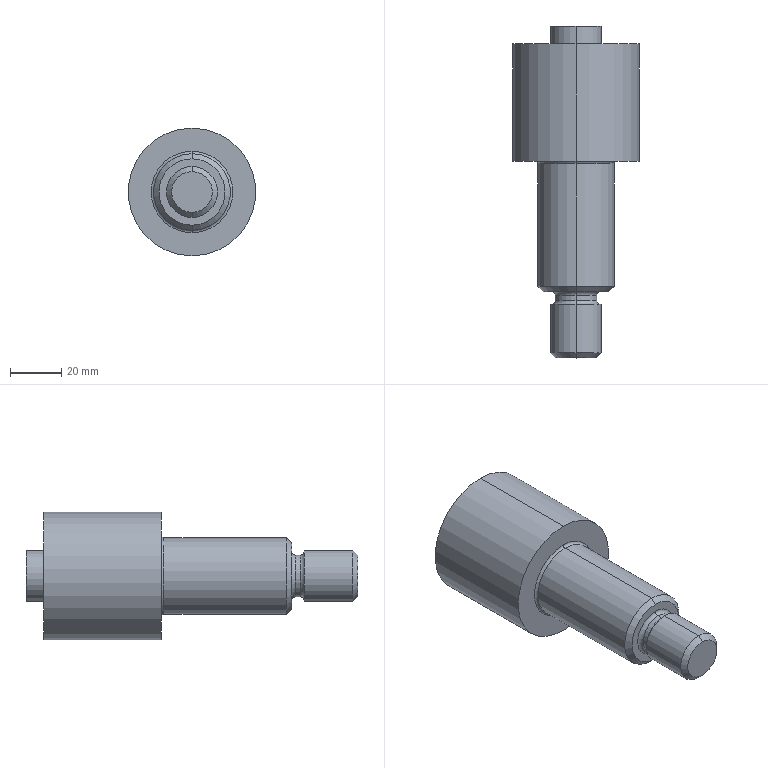Part | SolidWorks | features MirrorStock 1 | 1 solid | 26 faces | box 50 x 130 x 50 mm | volume 135954 mm3 | cylinder 10 | torus 6 | plane 6 | cone 4 | commonest cylinder face diameters 16.4 x2 19.8 x2 20 x2 30 x2 50 x2
STEP:
#1=CARTESIAN_POINT('',(0.,-107.5,-8.2));
#2=VERTEX_POINT('',#1);
#3=CARTESIAN_POINT('',(0.,-107.5,8.2));
#4=VERTEX_POINT('',#3);
#5=CARTESIAN_POINT('',(0.,-107.5,0.));
#6=DIRECTION('',(0.,-1.,0.));
#7=DIRECTION('',(0.,0.,-1.));
#8=AXIS2_PLACEMENT_3D('',#5,#6,#7);
#9=CIRCLE('',#8,8.2);
#10=EDGE_CURVE('',#2,#4,#9,.T.);
#11=ORIENTED_EDGE('',*,*,#10,.T.);
#12=CARTESIAN_POINT('',(0.,-109.,9.7));
#13=VERTEX_POINT('',#12);
#14=CARTESIAN_POINT('',(0.,-107.5,9.7));
#15=DIRECTION('',(-1.,0.,0.));
#16=DIRECTION('',(0.,0.,1.));
#17=AXIS2_PLACEMENT_3D('',#14,#15,#16);
#18=CIRCLE('',#17,1.5);
#19=EDGE_CURVE('',#4,#13,#18,.T.);
#20=ORIENTED_EDGE('',*,*,#19,.T.);
#21=CARTESIAN_POINT('',(0.,-109.,-9.7));
#22=VERTEX_POINT('',#21);
#23=CARTESIAN_POINT('',(0.,-109.,0.));
#24=DIRECTION('',(0.,1.,0.));
#25=DIRECTION('',(0.,0.,-1.));
#26=AXIS2_PLACEMENT_3D('',#23,#24,#25);
#27=CIRCLE('',#26,9.7);
#28=EDGE_CURVE('',#13,#22,#27,.T.);
#29=ORIENTED_EDGE('',*,*,#28,.T.);
#30=CARTESIAN_POINT('',(0.,-107.5,-9.7));
#31=DIRECTION('',(1.,0.,0.));
#32=DIRECTION('',(0.,0.,-1.));
#33=AXIS2_PLACEMENT_3D('',#30,#31,#32);
#34=CIRCLE('',#33,1.5);
#35=EDGE_CURVE('',#2,#22,#34,.T.);
#36=ORIENTED_EDGE('',*,*,#35,.F.);
#37=EDGE_LOOP('',(#11,#20,#29,#36));
#38=FACE_OUTER_BOUND('',#37,.T.);
#39=CARTESIAN_POINT('',(0.,-107.5,0.));
#40=DIRECTION('',(0.,1.,0.));
#41=DIRECTION('',(0.,0.,-1.));
#42=AXIS2_PLACEMENT_3D('',#39,#40,#41);
#43=TOROIDAL_SURFACE('',#42,9.7,1.5);
#44=ADVANCED_FACE('',(#38),#43,.F.);
#45=CARTESIAN_POINT('',(0.,-105.5,8.2));
#46=VERTEX_POINT('',#45);
#47=CARTESIAN_POINT('',(0.,-105.5,-8.2));
#48=VERTEX_POINT('',#47);
#49=CARTESIAN_POINT('',(0.,-105.5,0.));
#50=DIRECTION('',(0.,1.,0.));
#51=DIRECTION('',(0.,0.,1.));
#52=AXIS2_PLACEMENT_3D('',#49,#50,#51);
#53=CIRCLE('',#52,8.2);
#54=EDGE_CURVE('',#46,#48,#53,.T.);
#55=ORIENTED_EDGE('',*,*,#54,.T.);
#56=CARTESIAN_POINT('',(0.,-104.,-9.7));
#57=VERTEX_POINT('',#56);
#58=CARTESIAN_POINT('',(0.,-105.5,-9.7));
#59=DIRECTION('',(-1.,0.,0.));
#60=DIRECTION('',(0.,0.,1.));
#61=AXIS2_PLACEMENT_3D('',#58,#59,#60);
#62=CIRCLE('',#61,1.5);
#63=EDGE_CURVE('',#48,#57,#62,.T.);
#64=ORIENTED_EDGE('',*,*,#63,.T.);
#65=CARTESIAN_POINT('',(0.,-104.,9.7));
#66=VERTEX_POINT('',#65);
#67=CARTESIAN_POINT('',(0.,-104.,0.));
#68=DIRECTION('',(0.,-1.,0.));
#69=DIRECTION('',(0.,0.,1.));
#70=AXIS2_PLACEMENT_3D('',#67,#68,#69);
#71=CIRCLE('',#70,9.7);
#72=EDGE_CURVE('',#57,#66,#71,.T.);
#73=ORIENTED_EDGE('',*,*,#72,.T.);
#74=CARTESIAN_POINT('',(0.,-105.5,9.7));
#75=DIRECTION('',(1.,0.,0.));
#76=DIRECTION('',(0.,0.,-1.));
#77=AXIS2_PLACEMENT_3D('',#74,#75,#76);
#78=CIRCLE('',#77,1.5);
#79=EDGE_CURVE('',#46,#66,#78,.T.);
#80=ORIENTED_EDGE('',*,*,#79,.F.);
#81=EDGE_LOOP('',(#55,#64,#73,#80));
#82=FACE_OUTER_BOUND('',#81,.T.);
#83=CARTESIAN_POINT('',(0.,-105.5,0.));
#84=DIRECTION('',(0.,-1.,0.));
#85=DIRECTION('',(0.,0.,1.));
#86=AXIS2_PLACEMENT_3D('',#83,#84,#85);
#87=TOROIDAL_SURFACE('',#86,9.7,1.5);
#88=ADVANCED_FACE('',(#82),#87,.F.);
#89=CARTESIAN_POINT('',(0.,-54.,15.));
#90=VERTEX_POINT('',#89);
#91=CARTESIAN_POINT('',(0.,-54.,-15.));
#92=VERTEX_POINT('',#91);
#93=CARTESIAN_POINT('',(0.,-54.,0.));
#94=DIRECTION('',(0.,1.,0.));
#95=DIRECTION('',(0.,0.,1.));
#96=AXIS2_PLACEMENT_3D('',#93,#94,#95);
#97=CIRCLE('',#96,15.);
#98=EDGE_CURVE('',#90,#92,#97,.T.);
#99=ORIENTED_EDGE('',*,*,#98,.T.);
#100=CARTESIAN_POINT('',(0.,-53.,-16.));
#101=VERTEX_POINT('',#100);
#102=CARTESIAN_POINT('',(0.,-54.,-16.));
#103=DIRECTION('',(-1.,0.,0.));
#104=DIRECTION('',(0.,0.,1.));
#105=AXIS2_PLACEMENT_3D('',#102,#103,#104);
#106=CIRCLE('',#105,1.);
#107=EDGE_CURVE('',#92,#101,#106,.T.);
#108=ORIENTED_EDGE('',*,*,#107,.T.);
#109=CARTESIAN_POINT('',(0.,-53.,16.));
#110=VERTEX_POINT('',#109);
#111=CARTESIAN_POINT('',(0.,-53.,0.));
#112=DIRECTION('',(0.,-1.,0.));
#113=DIRECTION('',(0.,0.,1.));
#114=AXIS2_PLACEMENT_3D('',#111,#112,#113);
#115=CIRCLE('',#114,16.);
#116=EDGE_CURVE('',#101,#110,#115,.T.);
#117=ORIENTED_EDGE('',*,*,#116,.T.);
#118=CARTESIAN_POINT('',(0.,-54.,16.));
#119=DIRECTION('',(1.,0.,0.));
#120=DIRECTION('',(0.,0.,-1.));
#121=AXIS2_PLACEMENT_3D('',#118,#119,#120);
#122=CIRCLE('',#121,1.);
#123=EDGE_CURVE('',#90,#110,#122,.T.);
#124=ORIENTED_EDGE('',*,*,#123,.F.);
#125=EDGE_LOOP('',(#99,#108,#117,#124));
#126=FACE_OUTER_BOUND('',#125,.T.);
#127=CARTESIAN_POINT('',(0.,-54.,0.));
#128=DIRECTION('',(0.,-1.,0.));
#129=DIRECTION('',(0.,0.,1.));
#130=AXIS2_PLACEMENT_3D('',#127,#128,#129);
#131=TOROIDAL_SURFACE('',#130,16.,1.);
#132=ADVANCED_FACE('',(#126),#131,.F.);
#133=CARTESIAN_POINT('',(0.,-130.,-8.));
#134=VERTEX_POINT('',#133);
#135=CARTESIAN_POINT('',(0.,-130.,8.));
#136=VERTEX_POINT('',#135);
#137=CARTESIAN_POINT('',(0.,-130.,0.));
#138=DIRECTION('',(0.,1.,0.));
#139=DIRECTION('',(0.,0.,1.));
#140=AXIS2_PLACEMENT_3D('',#137,#138,#139);
#141=CIRCLE('',#140,8.);
#142=EDGE_CURVE('',#134,#136,#141,.T.);
#143=ORIENTED_EDGE('',*,*,#142,.T.);
#144=CARTESIAN_POINT('',(0.,-128.,10.));
#145=VERTEX_POINT('',#144);
#146=CARTESIAN_POINT('',(0.,-130.,8.));
#147=DIRECTION('',(0.,0.7071,0.7071));
#148=VECTOR('',#147,1000.);
#149=LINE('',#146,#148);
#150=EDGE_CURVE('',#136,#145,#149,.T.);
#151=ORIENTED_EDGE('',*,*,#150,.T.);
#152=CARTESIAN_POINT('',(0.,-128.,-10.));
#153=VERTEX_POINT('',#152);
#154=CARTESIAN_POINT('',(0.,-128.,0.));
#155=DIRECTION('',(0.,-1.,0.));
#156=DIRECTION('',(0.,0.,1.));
#157=AXIS2_PLACEMENT_3D('',#154,#155,#156);
#158=CIRCLE('',#157,10.);
#159=EDGE_CURVE('',#145,#153,#158,.T.);
#160=ORIENTED_EDGE('',*,*,#159,.T.);
#161=CARTESIAN_POINT('',(0.,-130.,-8.));
#162=DIRECTION('',(0.,0.7071,-0.7071));
#163=VECTOR('',#162,1000.);
#164=LINE('',#161,#163);
#165=EDGE_CURVE('',#134,#153,#164,.T.);
#166=ORIENTED_EDGE('',*,*,#165,.F.);
#167=EDGE_LOOP('',(#143,#151,#160,#166));
#168=FACE_OUTER_BOUND('',#167,.T.);
#169=CARTESIAN_POINT('',(0.,-130.,0.));
#170=DIRECTION('',(0.,1.,0.));
#171=DIRECTION('',(0.,0.,-1.));
#172=AXIS2_PLACEMENT_3D('',#169,#170,#171);
#173=CONICAL_SURFACE('',#172,8.,0.7854);
#174=ADVANCED_FACE('',(#168),#173,.T.);
#175=CARTESIAN_POINT('',(0.,-104.,-13.));
#176=VERTEX_POINT('',#175);
#177=CARTESIAN_POINT('',(0.,-104.,13.));
#178=VERTEX_POINT('',#177);
#179=CARTESIAN_POINT('',(0.,-104.,0.));
#180=DIRECTION('',(0.,1.,0.));
#181=DIRECTION('',(0.,0.,1.));
#182=AXIS2_PLACEMENT_3D('',#179,#180,#181);
#183=CIRCLE('',#182,13.);
#184=EDGE_CURVE('',#176,#178,#183,.T.);
#185=ORIENTED_EDGE('',*,*,#184,.T.);
#186=CARTESIAN_POINT('',(0.,-102.,15.));
#187=VERTEX_POINT('',#186);
#188=CARTESIAN_POINT('',(0.,-104.,13.));
#189=DIRECTION('',(0.,0.7071,0.7071));
#190=VECTOR('',#189,1000.);
#191=LINE('',#188,#190);
#192=EDGE_CURVE('',#178,#187,#191,.T.);
#193=ORIENTED_EDGE('',*,*,#192,.T.);
#194=CARTESIAN_POINT('',(0.,-102.,-15.));
#195=VERTEX_POINT('',#194);
#196=CARTESIAN_POINT('',(0.,-102.,0.));
#197=DIRECTION('',(0.,-1.,0.));
#198=DIRECTION('',(0.,0.,1.));
#199=AXIS2_PLACEMENT_3D('',#196,#197,#198);
#200=CIRCLE('',#199,15.);
#201=EDGE_CURVE('',#187,#195,#200,.T.);
#202=ORIENTED_EDGE('',*,*,#201,.T.);
#203=CARTESIAN_POINT('',(0.,-104.,-13.));
#204=DIRECTION('',(0.,0.7071,-0.7071));
#205=VECTOR('',#204,1000.);
#206=LINE('',#203,#205);
#207=EDGE_CURVE('',#176,#195,#206,.T.);
#208=ORIENTED_EDGE('',*,*,#207,.F.);
#209=EDGE_LOOP('',(#185,#193,#202,#208));
#210=FACE_OUTER_BOUND('',#209,.T.);
#211=CARTESIAN_POINT('',(0.,-104.,0.));
#212=DIRECTION('',(0.,1.,0.));
#213=DIRECTION('',(0.,0.,-1.));
#214=AXIS2_PLACEMENT_3D('',#211,#212,#213);
#215=CONICAL_SURFACE('',#214,13.,0.7854);
#216=ADVANCED_FACE('',(#210),#215,.T.);
#217=CARTESIAN_POINT('',(0.,-109.,-10.));
#218=VERTEX_POINT('',#217);
#219=CARTESIAN_POINT('',(0.,-109.,10.));
#220=VERTEX_POINT('',#219);
#221=CARTESIAN_POINT('',(0.,-109.,0.));
#222=DIRECTION('',(0.,1.,0.));
#223=DIRECTION('',(0.,0.,1.));
#224=AXIS2_PLACEMENT_3D('',#221,#222,#223);
#225=CIRCLE('',#224,10.);
#226=EDGE_CURVE('',#218,#220,#225,.T.);
#227=ORIENTED_EDGE('',*,*,#226,.F.);
#228=CARTESIAN_POINT('',(0.,-130.,-10.));
#229=DIRECTION('',(0.,-1.,0.));
#230=VECTOR('',#229,1000.);
#231=LINE('',#228,#230);
#232=EDGE_CURVE('',#218,#153,#231,.T.);
#233=ORIENTED_EDGE('',*,*,#232,.T.);
#234=ORIENTED_EDGE('',*,*,#159,.F.);
#235=CARTESIAN_POINT('',(0.,-130.,10.));
#236=DIRECTION('',(0.,-1.,0.));
#237=VECTOR('',#236,1000.);
#238=LINE('',#235,#237);
#239=EDGE_CURVE('',#220,#145,#238,.T.);
#240=ORIENTED_EDGE('',*,*,#239,.F.);
#241=EDGE_LOOP('',(#227,#233,#234,#240));
#242=FACE_OUTER_BOUND('',#241,.T.);
#243=CARTESIAN_POINT('',(0.,-130.,0.));
#244=DIRECTION('',(0.,-1.,0.));
#245=DIRECTION('',(0.,0.,1.));
#246=AXIS2_PLACEMENT_3D('',#243,#244,#245);
#247=CYLINDRICAL_SURFACE('',#246,10.);
#248=ADVANCED_FACE('',(#242),#247,.T.);
#249=CARTESIAN_POINT('',(0.,-105.5,0.));
#250=DIRECTION('',(0.,1.,0.));
#251=DIRECTION('',(0.,0.,1.));
#252=AXIS2_PLACEMENT_3D('',#249,#250,#251);
#253=CIRCLE('',#252,8.2);
#254=EDGE_CURVE('',#48,#46,#253,.T.);
#255=ORIENTED_EDGE('',*,*,#254,.F.);
#256=CARTESIAN_POINT('',(0.,-130.,-8.2));
#257=DIRECTION('',(0.,-1.,0.));
#258=VECTOR('',#257,1000.);
#259=LINE('',#256,#258);
#260=EDGE_CURVE('',#48,#2,#259,.T.);
#261=ORIENTED_EDGE('',*,*,#260,.T.);
#262=CARTESIAN_POINT('',(0.,-107.5,0.));
#263=DIRECTION('',(0.,-1.,0.));
#264=DIRECTION('',(0.,0.,-1.));
#265=AXIS2_PLACEMENT_3D('',#262,#263,#264);
#266=CIRCLE('',#265,8.2);
#267=EDGE_CURVE('',#4,#2,#266,.T.);
#268=ORIENTED_EDGE('',*,*,#267,.F.);
#269=CARTESIAN_POINT('',(0.,-130.,8.2));
#270=DIRECTION('',(0.,-1.,0.));
#271=VECTOR('',#270,1000.);
#272=LINE('',#269,#271);
#273=EDGE_CURVE('',#46,#4,#272,.T.);
#274=ORIENTED_EDGE('',*,*,#273,.F.);
#275=EDGE_LOOP('',(#255,#261,#268,#274));
#276=FACE_OUTER_BOUND('',#275,.T.);
#277=CARTESIAN_POINT('',(0.,-130.,0.));
#278=DIRECTION('',(0.,-1.,0.));
#279=DIRECTION('',(0.,0.,1.));
#280=AXIS2_PLACEMENT_3D('',#277,#278,#279);
#281=CYLINDRICAL_SURFACE('',#280,8.2);
#282=ADVANCED_FACE('',(#276),#281,.T.);
#283=CARTESIAN_POINT('',(0.,-54.,0.));
#284=DIRECTION('',(0.,1.,0.));
#285=DIRECTION('',(0.,0.,1.));
#286=AXIS2_PLACEMENT_3D('',#283,#284,#285);
#287=CIRCLE('',#286,15.);
#288=EDGE_CURVE('',#92,#90,#287,.T.);
#289=ORIENTED_EDGE('',*,*,#288,.F.);
#290=CARTESIAN_POINT('',(0.,-130.,-15.));
#291=DIRECTION('',(0.,-1.,0.));
#292=VECTOR('',#291,1000.);
#293=LINE('',#290,#292);
#294=EDGE_CURVE('',#92,#195,#293,.T.);
#295=ORIENTED_EDGE('',*,*,#294,.T.);
#296=ORIENTED_EDGE('',*,*,#201,.F.);
#297=CARTESIAN_POINT('',(0.,-130.,15.));
#298=DIRECTION('',(0.,-1.,0.));
#299=VECTOR('',#298,1000.);
#300=LINE('',#297,#299);
#301=EDGE_CURVE('',#90,#187,#300,.T.);
#302=ORIENTED_EDGE('',*,*,#301,.F.);
#303=EDGE_LOOP('',(#289,#295,#296,#302));
#304=FACE_OUTER_BOUND('',#303,.T.);
#305=CARTESIAN_POINT('',(0.,-130.,0.));
#306=DIRECTION('',(0.,-1.,0.));
#307=DIRECTION('',(0.,0.,1.));
#308=AXIS2_PLACEMENT_3D('',#305,#306,#307);
#309=CYLINDRICAL_SURFACE('',#308,15.);
#310=ADVANCED_FACE('',(#304),#309,.T.);
#311=CARTESIAN_POINT('',(0.,-7.,-25.));
#312=VERTEX_POINT('',#311);
#313=CARTESIAN_POINT('',(0.,-7.,25.));
#314=VERTEX_POINT('',#313);
#315=CARTESIAN_POINT('',(0.,-7.,0.));
#316=DIRECTION('',(0.,1.,0.));
#317=DIRECTION('',(0.,0.,1.));
#318=AXIS2_PLACEMENT_3D('',#315,#316,#317);
#319=CIRCLE('',#318,25.);
#320=EDGE_CURVE('',#312,#314,#319,.T.);
#321=ORIENTED_EDGE('',*,*,#320,.F.);
#322=CARTESIAN_POINT('',(0.,-53.,-25.));
#323=VERTEX_POINT('',#322);
#324=CARTESIAN_POINT('',(0.,-130.,-25.));
#325=DIRECTION('',(0.,-1.,0.));
#326=VECTOR('',#325,1000.);
#327=LINE('',#324,#326);
#328=EDGE_CURVE('',#312,#323,#327,.T.);
#329=ORIENTED_EDGE('',*,*,#328,.T.);
#330=CARTESIAN_POINT('',(0.,-53.,25.));
#331=VERTEX_POINT('',#330);
#332=CARTESIAN_POINT('',(0.,-53.,0.));
#333=DIRECTION('',(0.,1.,0.));
#334=DIRECTION('',(0.,0.,1.));
#335=AXIS2_PLACEMENT_3D('',#332,#333,#334);
#336=CIRCLE('',#335,25.);
#337=EDGE_CURVE('',#323,#331,#336,.T.);
#338=ORIENTED_EDGE('',*,*,#337,.T.);
#339=CARTESIAN_POINT('',(0.,-130.,25.));
#340=DIRECTION('',(0.,-1.,0.));
#341=VECTOR('',#340,1000.);
#342=LINE('',#339,#341);
#343=EDGE_CURVE('',#314,#331,#342,.T.);
#344=ORIENTED_EDGE('',*,*,#343,.F.);
#345=EDGE_LOOP('',(#321,#329,#338,#344));
#346=FACE_OUTER_BOUND('',#345,.T.);
#347=CARTESIAN_POINT('',(0.,-130.,0.));
#348=DIRECTION('',(0.,-1.,0.));
#349=DIRECTION('',(0.,0.,1.));
#350=AXIS2_PLACEMENT_3D('',#347,#348,#349);
#351=CYLINDRICAL_SURFACE('',#350,25.);
#352=ADVANCED_FACE('',(#346),#351,.T.);
#353=CARTESIAN_POINT('',(0.,0.,-9.9));
#354=VERTEX_POINT('',#353);
#355=CARTESIAN_POINT('',(0.,0.,9.9));
#356=VERTEX_POINT('',#355);
#357=CARTESIAN_POINT('',(0.,0.,0.));
#358=DIRECTION('',(0.,1.,0.));
#359=DIRECTION('',(0.,0.,1.));
#360=AXIS2_PLACEMENT_3D('',#357,#358,#359);
#361=CIRCLE('',#360,9.9);
#362=EDGE_CURVE('',#354,#356,#361,.T.);
#363=ORIENTED_EDGE('',*,*,#362,.F.);
#364=CARTESIAN_POINT('',(0.,-7.,-9.9));
#365=VERTEX_POINT('',#364);
#366=CARTESIAN_POINT('',(0.,-130.,-9.9));
#367=DIRECTION('',(0.,-1.,0.));
#368=VECTOR('',#367,1000.);
#369=LINE('',#366,#368);
#370=EDGE_CURVE('',#354,#365,#369,.T.);
#371=ORIENTED_EDGE('',*,*,#370,.T.);
#372=CARTESIAN_POINT('',(0.,-7.,9.9));
#373=VERTEX_POINT('',#372);
#374=CARTESIAN_POINT('',(0.,-7.,0.));
#375=DIRECTION('',(0.,1.,0.));
#376=DIRECTION('',(0.,0.,1.));
#377=AXIS2_PLACEMENT_3D('',#374,#375,#376);
#378=CIRCLE('',#377,9.9);
#379=EDGE_CURVE('',#365,#373,#378,.T.);
#380=ORIENTED_EDGE('',*,*,#379,.T.);
#381=CARTESIAN_POINT('',(0.,-130.,9.9));
#382=DIRECTION('',(0.,-1.,0.));
#383=VECTOR('',#382,1000.);
#384=LINE('',#381,#383);
#385=EDGE_CURVE('',#356,#373,#384,.T.);
#386=ORIENTED_EDGE('',*,*,#385,.F.);
#387=EDGE_LOOP('',(#363,#371,#380,#386));
#388=FACE_OUTER_BOUND('',#387,.T.);
#389=CARTESIAN_POINT('',(0.,-130.,0.));
#390=DIRECTION('',(0.,-1.,0.));
#391=DIRECTION('',(0.,0.,1.));
#392=AXIS2_PLACEMENT_3D('',#389,#390,#391);
#393=CYLINDRICAL_SURFACE('',#392,9.9);
#394=ADVANCED_FACE('',(#388),#393,.T.);
#395=CARTESIAN_POINT('',(0.,0.,0.));
#396=DIRECTION('',(0.,1.,0.));
#397=DIRECTION('',(0.,0.,1.));
#398=AXIS2_PLACEMENT_3D('',#395,#396,#397);
#399=CIRCLE('',#398,9.9);
#400=EDGE_CURVE('',#356,#354,#399,.T.);
#401=ORIENTED_EDGE('',*,*,#400,.T.);
#402=ORIENTED_EDGE('',*,*,#362,.T.);
#403=EDGE_LOOP('',(#401,#402));
#404=FACE_OUTER_BOUND('',#403,.T.);
#405=CARTESIAN_POINT('',(0.,0.,0.));
#406=DIRECTION('',(0.,1.,0.));
#407=DIRECTION('',(0.,0.,-1.));
#408=AXIS2_PLACEMENT_3D('',#405,#406,#407);
#409=PLANE('',#408);
#410=ADVANCED_FACE('',(#404),#409,.T.);
#411=ORIENTED_EDGE('',*,*,#370,.F.);
#412=ORIENTED_EDGE('',*,*,#400,.F.);
#413=ORIENTED_EDGE('',*,*,#385,.T.);
#414=CARTESIAN_POINT('',(0.,-7.,0.));
#415=DIRECTION('',(0.,1.,0.));
#416=DIRECTION('',(0.,0.,1.));
#417=AXIS2_PLACEMENT_3D('',#414,#415,#416);
#418=CIRCLE('',#417,9.9);
#419=EDGE_CURVE('',#373,#365,#418,.T.);
#420=ORIENTED_EDGE('',*,*,#419,.T.);
#421=EDGE_LOOP('',(#411,#412,#413,#420));
#422=FACE_OUTER_BOUND('',#421,.T.);
#423=CARTESIAN_POINT('',(0.,-130.,0.));
#424=DIRECTION('',(0.,-1.,0.));
#425=DIRECTION('',(0.,0.,1.));
#426=AXIS2_PLACEMENT_3D('',#423,#424,#425);
#427=CYLINDRICAL_SURFACE('',#426,9.9);
#428=ADVANCED_FACE('',(#422),#427,.T.);
#429=ORIENTED_EDGE('',*,*,#419,.F.);
#430=ORIENTED_EDGE('',*,*,#379,.F.);
#431=EDGE_LOOP('',(#429,#430));
#432=FACE_BOUND('',#431,.T.);
#433=CARTESIAN_POINT('',(0.,-7.,0.));
#434=DIRECTION('',(0.,1.,0.));
#435=DIRECTION('',(0.,0.,1.));
#436=AXIS2_PLACEMENT_3D('',#433,#434,#435);
#437=CIRCLE('',#436,25.);
#438=EDGE_CURVE('',#314,#312,#437,.T.);
#439=ORIENTED_EDGE('',*,*,#438,.T.);
#440=ORIENTED_EDGE('',*,*,#320,.T.);
#441=EDGE_LOOP('',(#439,#440));
#442=FACE_OUTER_BOUND('',#441,.T.);
#443=CARTESIAN_POINT('',(9.9,-7.,0.));
#444=DIRECTION('',(0.,1.,0.));
#445=DIRECTION('',(0.,0.,-1.));
#446=AXIS2_PLACEMENT_3D('',#443,#444,#445);
#447=PLANE('',#446);
#448=ADVANCED_FACE('',(#432,#442),#447,.T.);
#449=ORIENTED_EDGE('',*,*,#328,.F.);
#450=ORIENTED_EDGE('',*,*,#438,.F.);
#451=ORIENTED_EDGE('',*,*,#343,.T.);
#452=CARTESIAN_POINT('',(0.,-53.,0.));
#453=DIRECTION('',(0.,1.,0.));
#454=DIRECTION('',(0.,0.,1.));
#455=AXIS2_PLACEMENT_3D('',#452,#453,#454);
#456=CIRCLE('',#455,25.);
#457=EDGE_CURVE('',#331,#323,#456,.T.);
#458=ORIENTED_EDGE('',*,*,#457,.T.);
#459=EDGE_LOOP('',(#449,#450,#451,#458));
#460=FACE_OUTER_BOUND('',#459,.T.);
#461=CARTESIAN_POINT('',(0.,-130.,0.));
#462=DIRECTION('',(0.,-1.,0.));
#463=DIRECTION('',(0.,0.,1.));
#464=AXIS2_PLACEMENT_3D('',#461,#462,#463);
#465=CYLINDRICAL_SURFACE('',#464,25.);
#466=ADVANCED_FACE('',(#460),#465,.T.);
#467=CARTESIAN_POINT('',(0.,-53.,0.));
#468=DIRECTION('',(0.,-1.,0.));
#469=DIRECTION('',(0.,0.,1.));
#470=AXIS2_PLACEMENT_3D('',#467,#468,#469);
#471=CIRCLE('',#470,16.);
#472=EDGE_CURVE('',#110,#101,#471,.T.);
#473=ORIENTED_EDGE('',*,*,#472,.F.);
#474=ORIENTED_EDGE('',*,*,#116,.F.);
#475=EDGE_LOOP('',(#473,#474));
#476=FACE_BOUND('',#475,.T.);
#477=ORIENTED_EDGE('',*,*,#457,.F.);
#478=ORIENTED_EDGE('',*,*,#337,.F.);
#479=EDGE_LOOP('',(#477,#478));
#480=FACE_OUTER_BOUND('',#479,.T.);
#481=CARTESIAN_POINT('',(25.,-53.,0.));
#482=DIRECTION('',(0.,-1.,0.));
#483=DIRECTION('',(0.,0.,1.));
#484=AXIS2_PLACEMENT_3D('',#481,#482,#483);
#485=PLANE('',#484);
#486=ADVANCED_FACE('',(#476,#480),#485,.T.);
#487=ORIENTED_EDGE('',*,*,#294,.F.);
#488=ORIENTED_EDGE('',*,*,#98,.F.);
#489=ORIENTED_EDGE('',*,*,#301,.T.);
#490=CARTESIAN_POINT('',(0.,-102.,0.));
#491=DIRECTION('',(0.,-1.,0.));
#492=DIRECTION('',(0.,0.,1.));
#493=AXIS2_PLACEMENT_3D('',#490,#491,#492);
#494=CIRCLE('',#493,15.);
#495=EDGE_CURVE('',#195,#187,#494,.T.);
#496=ORIENTED_EDGE('',*,*,#495,.F.);
#497=EDGE_LOOP('',(#487,#488,#489,#496));
#498=FACE_OUTER_BOUND('',#497,.T.);
#499=CARTESIAN_POINT('',(0.,-130.,0.));
#500=DIRECTION('',(0.,-1.,0.));
#501=DIRECTION('',(0.,0.,1.));
#502=AXIS2_PLACEMENT_3D('',#499,#500,#501);
#503=CYLINDRICAL_SURFACE('',#502,15.);
#504=ADVANCED_FACE('',(#498),#503,.T.);
#505=CARTESIAN_POINT('',(0.,-104.,0.));
#506=DIRECTION('',(0.,-1.,0.));
#507=DIRECTION('',(0.,0.,1.));
#508=AXIS2_PLACEMENT_3D('',#505,#506,#507);
#509=CIRCLE('',#508,9.7);
#510=EDGE_CURVE('',#66,#57,#509,.T.);
#511=ORIENTED_EDGE('',*,*,#510,.F.);
#512=ORIENTED_EDGE('',*,*,#72,.F.);
#513=EDGE_LOOP('',(#511,#512));
#514=FACE_BOUND('',#513,.T.);
#515=ORIENTED_EDGE('',*,*,#184,.F.);
#516=CARTESIAN_POINT('',(0.,-104.,0.));
#517=DIRECTION('',(0.,1.,0.));
#518=DIRECTION('',(0.,0.,1.));
#519=AXIS2_PLACEMENT_3D('',#516,#517,#518);
#520=CIRCLE('',#519,13.);
#521=EDGE_CURVE('',#178,#176,#520,.T.);
#522=ORIENTED_EDGE('',*,*,#521,.F.);
#523=EDGE_LOOP('',(#515,#522));
#524=FACE_OUTER_BOUND('',#523,.T.);
#525=CARTESIAN_POINT('',(15.,-104.,0.));
#526=DIRECTION('',(0.,-1.,0.));
#527=DIRECTION('',(0.,0.,1.));
#528=AXIS2_PLACEMENT_3D('',#525,#526,#527);
#529=PLANE('',#528);
#530=ADVANCED_FACE('',(#514,#524),#529,.T.);
#531=ORIENTED_EDGE('',*,*,#260,.F.);
#532=ORIENTED_EDGE('',*,*,#54,.F.);
#533=ORIENTED_EDGE('',*,*,#273,.T.);
#534=ORIENTED_EDGE('',*,*,#10,.F.);
#535=EDGE_LOOP('',(#531,#532,#533,#534));
#536=FACE_OUTER_BOUND('',#535,.T.);
#537=CARTESIAN_POINT('',(0.,-130.,0.));
#538=DIRECTION('',(0.,-1.,0.));
#539=DIRECTION('',(0.,0.,1.));
#540=AXIS2_PLACEMENT_3D('',#537,#538,#539);
#541=CYLINDRICAL_SURFACE('',#540,8.2);
#542=ADVANCED_FACE('',(#536),#541,.T.);
#543=CARTESIAN_POINT('',(0.,-109.,0.));
#544=DIRECTION('',(0.,1.,0.));
#545=DIRECTION('',(0.,0.,-1.));
#546=AXIS2_PLACEMENT_3D('',#543,#544,#545);
#547=CIRCLE('',#546,9.7);
#548=EDGE_CURVE('',#22,#13,#547,.T.);
#549=ORIENTED_EDGE('',*,*,#548,.F.);
#550=ORIENTED_EDGE('',*,*,#28,.F.);
#551=EDGE_LOOP('',(#549,#550));
#552=FACE_BOUND('',#551,.T.);
#553=CARTESIAN_POINT('',(0.,-109.,0.));
#554=DIRECTION('',(0.,1.,0.));
#555=DIRECTION('',(0.,0.,1.));
#556=AXIS2_PLACEMENT_3D('',#553,#554,#555);
#557=CIRCLE('',#556,10.);
#558=EDGE_CURVE('',#220,#218,#557,.T.);
#559=ORIENTED_EDGE('',*,*,#558,.T.);
#560=ORIENTED_EDGE('',*,*,#226,.T.);
#561=EDGE_LOOP('',(#559,#560));
#562=FACE_OUTER_BOUND('',#561,.T.);
#563=CARTESIAN_POINT('',(8.2,-109.,0.));
#564=DIRECTION('',(0.,1.,0.));
#565=DIRECTION('',(0.,0.,-1.));
#566=AXIS2_PLACEMENT_3D('',#563,#564,#565);
#567=PLANE('',#566);
#568=ADVANCED_FACE('',(#552,#562),#567,.T.);
#569=ORIENTED_EDGE('',*,*,#232,.F.);
#570=ORIENTED_EDGE('',*,*,#558,.F.);
#571=ORIENTED_EDGE('',*,*,#239,.T.);
#572=CARTESIAN_POINT('',(0.,-128.,0.));
#573=DIRECTION('',(0.,-1.,0.));
#574=DIRECTION('',(0.,0.,1.));
#575=AXIS2_PLACEMENT_3D('',#572,#573,#574);
#576=CIRCLE('',#575,10.);
#577=EDGE_CURVE('',#153,#145,#576,.T.);
#578=ORIENTED_EDGE('',*,*,#577,.F.);
#579=EDGE_LOOP('',(#569,#570,#571,#578));
#580=FACE_OUTER_BOUND('',#579,.T.);
#581=CARTESIAN_POINT('',(0.,-130.,0.));
#582=DIRECTION('',(0.,-1.,0.));
#583=DIRECTION('',(0.,0.,1.));
#584=AXIS2_PLACEMENT_3D('',#581,#582,#583);
#585=CYLINDRICAL_SURFACE('',#584,10.);
#586=ADVANCED_FACE('',(#580),#585,.T.);
#587=ORIENTED_EDGE('',*,*,#142,.F.);
#588=CARTESIAN_POINT('',(0.,-130.,0.));
#589=DIRECTION('',(0.,1.,0.));
#590=DIRECTION('',(0.,0.,1.));
#591=AXIS2_PLACEMENT_3D('',#588,#589,#590);
#592=CIRCLE('',#591,8.);
#593=EDGE_CURVE('',#136,#134,#592,.T.);
#594=ORIENTED_EDGE('',*,*,#593,.F.);
#595=EDGE_LOOP('',(#587,#594));
#596=FACE_OUTER_BOUND('',#595,.T.);
#597=CARTESIAN_POINT('',(10.,-130.,0.));
#598=DIRECTION('',(0.,-1.,0.));
#599=DIRECTION('',(0.,0.,1.));
#600=AXIS2_PLACEMENT_3D('',#597,#598,#599);
#601=PLANE('',#600);
#602=ADVANCED_FACE('',(#596),#601,.T.);
#603=ORIENTED_EDGE('',*,*,#192,.F.);
#604=ORIENTED_EDGE('',*,*,#521,.T.);
#605=ORIENTED_EDGE('',*,*,#207,.T.);
#606=ORIENTED_EDGE('',*,*,#495,.T.);
#607=EDGE_LOOP('',(#603,#604,#605,#606));
#608=FACE_OUTER_BOUND('',#607,.T.);
#609=CARTESIAN_POINT('',(0.,-104.,0.));
#610=DIRECTION('',(0.,1.,0.));
#611=DIRECTION('',(0.,0.,-1.));
#612=AXIS2_PLACEMENT_3D('',#609,#610,#611);
#613=CONICAL_SURFACE('',#612,13.,0.7854);
#614=ADVANCED_FACE('',(#608),#613,.T.);
#615=ORIENTED_EDGE('',*,*,#150,.F.);
#616=ORIENTED_EDGE('',*,*,#593,.T.);
#617=ORIENTED_EDGE('',*,*,#165,.T.);
#618=ORIENTED_EDGE('',*,*,#577,.T.);
#619=EDGE_LOOP('',(#615,#616,#617,#618));
#620=FACE_OUTER_BOUND('',#619,.T.);
#621=CARTESIAN_POINT('',(0.,-130.,0.));
#622=DIRECTION('',(0.,1.,0.));
#623=DIRECTION('',(0.,0.,-1.));
#624=AXIS2_PLACEMENT_3D('',#621,#622,#623);
#625=CONICAL_SURFACE('',#624,8.,0.7854);
#626=ADVANCED_FACE('',(#620),#625,.T.);
#627=ORIENTED_EDGE('',*,*,#107,.F.);
#628=ORIENTED_EDGE('',*,*,#288,.T.);
#629=ORIENTED_EDGE('',*,*,#123,.T.);
#630=ORIENTED_EDGE('',*,*,#472,.T.);
#631=EDGE_LOOP('',(#627,#628,#629,#630));
#632=FACE_OUTER_BOUND('',#631,.T.);
#633=CARTESIAN_POINT('',(0.,-54.,0.));
#634=DIRECTION('',(0.,-1.,0.));
#635=DIRECTION('',(0.,0.,1.));
#636=AXIS2_PLACEMENT_3D('',#633,#634,#635);
#637=TOROIDAL_SURFACE('',#636,16.,1.);
#638=ADVANCED_FACE('',(#632),#637,.F.);
#639=ORIENTED_EDGE('',*,*,#63,.F.);
#640=ORIENTED_EDGE('',*,*,#254,.T.);
#641=ORIENTED_EDGE('',*,*,#79,.T.);
#642=ORIENTED_EDGE('',*,*,#510,.T.);
#643=EDGE_LOOP('',(#639,#640,#641,#642));
#644=FACE_OUTER_BOUND('',#643,.T.);
#645=CARTESIAN_POINT('',(0.,-105.5,0.));
#646=DIRECTION('',(0.,-1.,0.));
#647=DIRECTION('',(0.,0.,1.));
#648=AXIS2_PLACEMENT_3D('',#645,#646,#647);
#649=TOROIDAL_SURFACE('',#648,9.7,1.5);
#650=ADVANCED_FACE('',(#644),#649,.F.);
#651=ORIENTED_EDGE('',*,*,#19,.F.);
#652=ORIENTED_EDGE('',*,*,#267,.T.);
#653=ORIENTED_EDGE('',*,*,#35,.T.);
#654=ORIENTED_EDGE('',*,*,#548,.T.);
#655=EDGE_LOOP('',(#651,#652,#653,#654));
#656=FACE_OUTER_BOUND('',#655,.T.);
#657=CARTESIAN_POINT('',(0.,-107.5,0.));
#658=DIRECTION('',(0.,1.,0.));
#659=DIRECTION('',(0.,0.,-1.));
#660=AXIS2_PLACEMENT_3D('',#657,#658,#659);
#661=TOROIDAL_SURFACE('',#660,9.7,1.5);
#662=ADVANCED_FACE('',(#656),#661,.F.);
#663=CLOSED_SHELL('',(#44,#88,#132,#174,#216,#248,#282,#310,#352,#394,#410,#428,#448,#466,#486,#504,#530,#542,#568,#586,#602,#614,#626,#638,#650,#662));
#664=MANIFOLD_SOLID_BREP('',#663);
#665=CARTESIAN_POINT('',(0.,0.,0.));
#666=DIRECTION('',(0.,0.,1.));
#667=DIRECTION('',(1.,0.,0.));
#668=AXIS2_PLACEMENT_3D('',#665,#666,#667);
#669=(LENGTH_UNIT()NAMED_UNIT(*)SI_UNIT(.MILLI.,.METRE.));
#670=UNCERTAINTY_MEASURE_WITH_UNIT(LENGTH_MEASURE(0.00001),#669,'','');
#671=(NAMED_UNIT(*)PLANE_ANGLE_UNIT()SI_UNIT($,.RADIAN.));
#672=(NAMED_UNIT(*)SI_UNIT($,.STERADIAN.)SOLID_ANGLE_UNIT());
#673=(GEOMETRIC_REPRESENTATION_CONTEXT(3)GLOBAL_UNCERTAINTY_ASSIGNED_CONTEXT((#670))GLOBAL_UNIT_ASSIGNED_CONTEXT((#669,#671,#672))REPRESENTATION_CONTEXT('',''));
#674=ADVANCED_BREP_SHAPE_REPRESENTATION('',(#664,#668),#673);